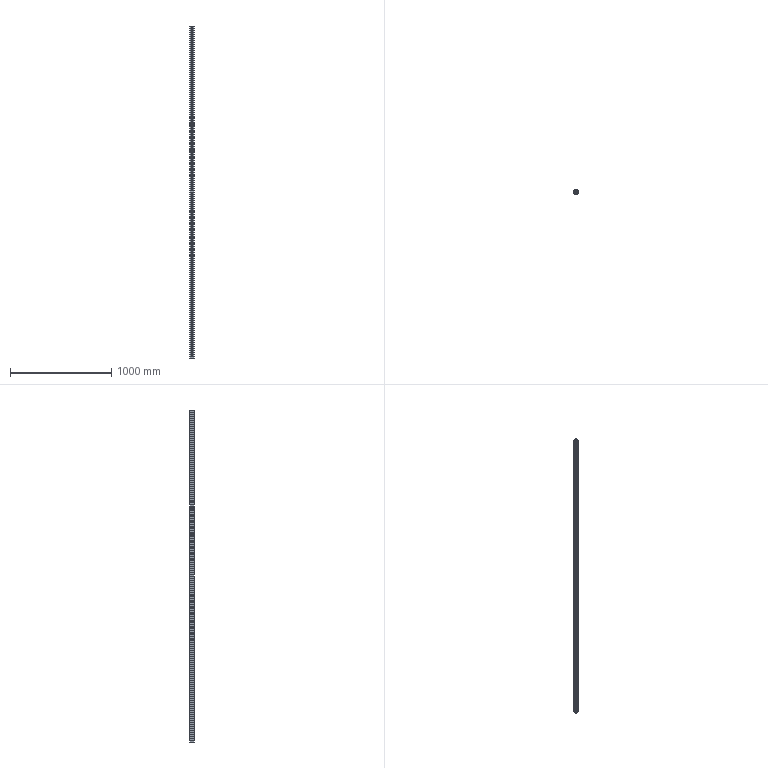Part | SolidWorks | features HoleWzd 2, Extrusion 1 | 1 solid | 309 faces | box 40 x 40 x 3280 mm | volume 1969669 mm3 | plane 211 | cylinder 98 | commonest cylinder face diameters 6.6 x40 11 x18 6.8 x15 1 x8 2 x8 5 x4